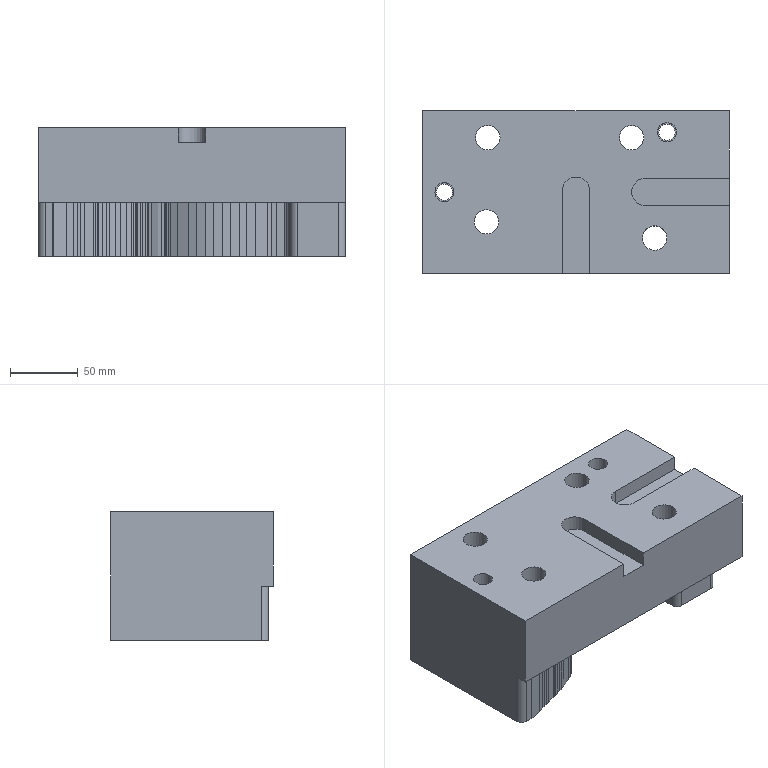Part | STEP file | lll_id3478_x_t | 1 solid | 113 faces | box 226 x 120 x 95 mm | volume 2052997 mm3 | plane 79 | cylinder 27 | cone 7 | commonest cylinder face diameters 10.506 x5 10 x4 18.009 x4 20 x4 26.007 x4 6.8 x2